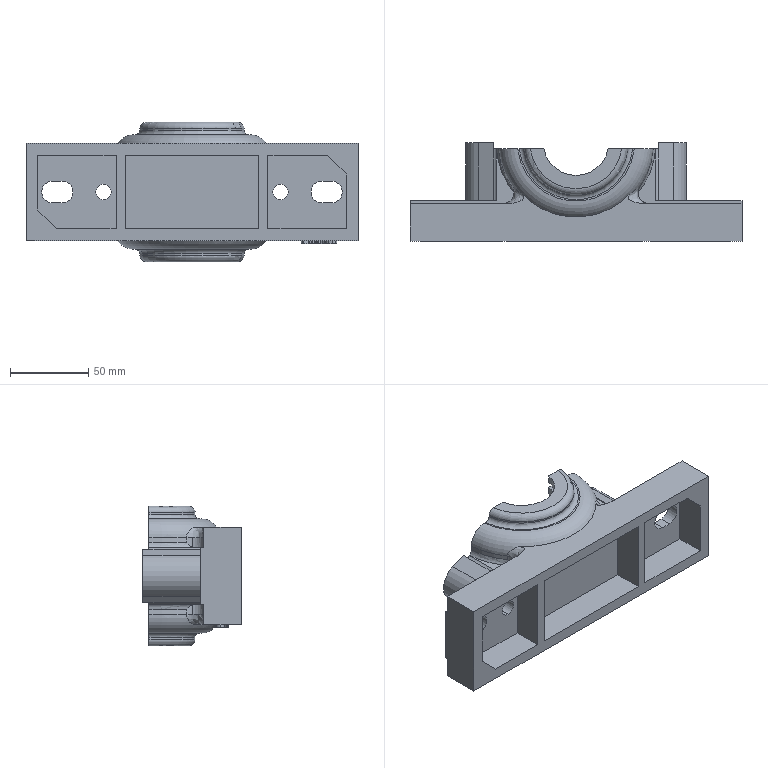Part | SolidWorks | features ICE 8, MirrorPattern 3, VarFillet 2, CombineBodies 1, MoveCopyBody 1, RevCut 1, Revolution 1, Stock 1 | 1 solid | 193 faces | box 212 x 63 x 89 mm | volume 297133 mm3 | spline 75 | plane 65 | cylinder 39 | torus 12 | cone 2 | commonest cylinder face diameters 14 x10 10 x8 42 x4 99 x4 113 x4 28 x2